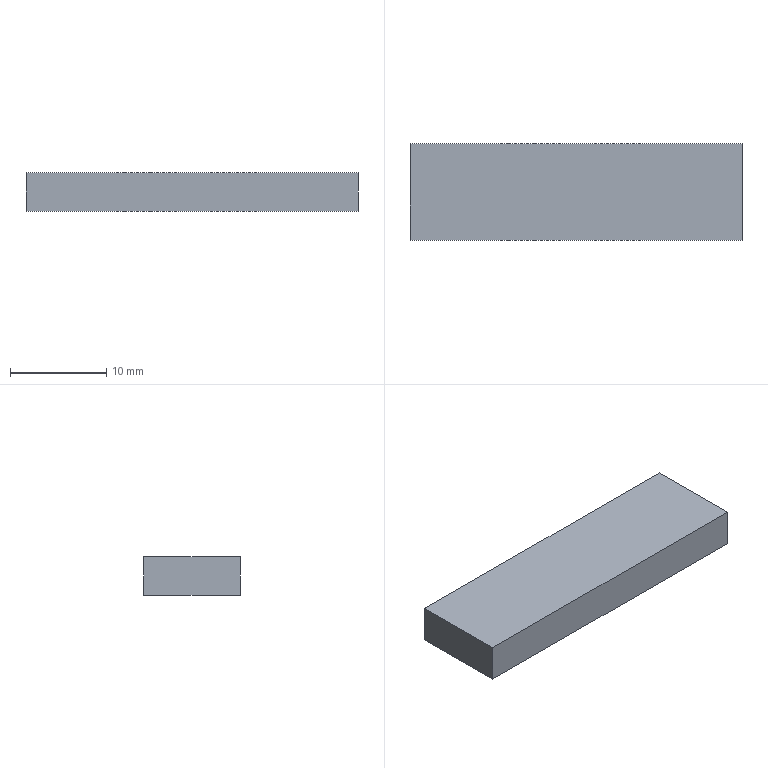Part | STEP file | YBQDJ-YB-30 | 1 solid | 6 faces | box 34.5 x 10 x 4 mm | volume 1380 mm3 | plane 6
STEP:
#1=CARTESIAN_POINT('',(0.,0.,0.));
#2=DIRECTION('',(0.,0.,1.));
#3=DIRECTION('',(1.,0.,0.));
#4=AXIS2_PLACEMENT_3D('',#1,#2,#3);
#5=CARTESIAN_POINT('',(-200.75,-276.,207.8));
#6=VERTEX_POINT('',#5);
#7=CARTESIAN_POINT('',(-200.75,-286.,207.8));
#8=VERTEX_POINT('',#7);
#9=CARTESIAN_POINT('',(-200.75,-276.,207.8));
#10=DIRECTION('',(0.,-1.,0.));
#11=VECTOR('',#10,1.);
#12=LINE('',#9,#11);
#13=CARTESIAN_POINT('',(-200.75,-276.,203.8));
#14=DIRECTION('',(-1.,0.,0.));
#15=DIRECTION('',(0.,0.,1.));
#16=AXIS2_PLACEMENT_3D('',#13,#14,#15);
#17=PLANE('',#16);
#18=CARTESIAN_POINT('',(4.,0.));
#19=DIRECTION('',(0.,-1.));
#20=VECTOR('',#19,1.);
#21=LINE('',#18,#20);
#22=(GEOMETRIC_REPRESENTATION_CONTEXT(2)PARAMETRIC_REPRESENTATION_CONTEXT()REPRESENTATION_CONTEXT('',''));
#23=DEFINITIONAL_REPRESENTATION('',(#21),#22);
#24=PCURVE('',#17,#23);
#25=CARTESIAN_POINT('',(0.,-172.,207.8));
#26=DIRECTION('',(0.,0.,1.));
#27=DIRECTION('',(1.,0.,0.));
#28=AXIS2_PLACEMENT_3D('',#25,#26,#27);
#29=PLANE('',#28);
#30=CARTESIAN_POINT('',(-200.75,-104.));
#31=DIRECTION('',(0.,-1.));
#32=VECTOR('',#31,1.);
#33=LINE('',#30,#32);
#34=(GEOMETRIC_REPRESENTATION_CONTEXT(2)PARAMETRIC_REPRESENTATION_CONTEXT()REPRESENTATION_CONTEXT('',''));
#35=DEFINITIONAL_REPRESENTATION('',(#33),#34);
#36=PCURVE('',#29,#35);
#37=SURFACE_CURVE('',#12,(#24,#36),.PCURVE_S1.);
#38=EDGE_CURVE('',#6,#8,#37,.T.);
#39=ORIENTED_EDGE('',*,*,#38,.F.);
#40=CARTESIAN_POINT('',(-200.75,-276.,203.8));
#41=VERTEX_POINT('',#40);
#42=CARTESIAN_POINT('',(-200.75,-276.,203.8));
#43=DIRECTION('',(0.,0.,1.));
#44=VECTOR('',#43,1.);
#45=LINE('',#42,#44);
#46=CARTESIAN_POINT('',(0.,0.));
#47=DIRECTION('',(1.,0.));
#48=VECTOR('',#47,1.);
#49=LINE('',#46,#48);
#50=(GEOMETRIC_REPRESENTATION_CONTEXT(2)PARAMETRIC_REPRESENTATION_CONTEXT()REPRESENTATION_CONTEXT('',''));
#51=DEFINITIONAL_REPRESENTATION('',(#49),#50);
#52=PCURVE('',#17,#51);
#53=CARTESIAN_POINT('',(-166.25,-276.,203.8));
#54=DIRECTION('',(0.,1.,0.));
#55=DIRECTION('',(0.,0.,1.));
#56=AXIS2_PLACEMENT_3D('',#53,#54,#55);
#57=PLANE('',#56);
#58=CARTESIAN_POINT('',(0.,-34.5));
#59=DIRECTION('',(1.,0.));
#60=VECTOR('',#59,1.);
#61=LINE('',#58,#60);
#62=(GEOMETRIC_REPRESENTATION_CONTEXT(2)PARAMETRIC_REPRESENTATION_CONTEXT()REPRESENTATION_CONTEXT('',''));
#63=DEFINITIONAL_REPRESENTATION('',(#61),#62);
#64=PCURVE('',#57,#63);
#65=SURFACE_CURVE('',#45,(#52,#64),.PCURVE_S1.);
#66=EDGE_CURVE('',#41,#6,#65,.T.);
#67=ORIENTED_EDGE('',*,*,#66,.F.);
#68=CARTESIAN_POINT('',(-200.75,-286.,203.8));
#69=VERTEX_POINT('',#68);
#70=CARTESIAN_POINT('',(-200.75,-276.,203.8));
#71=DIRECTION('',(0.,-1.,0.));
#72=VECTOR('',#71,1.);
#73=LINE('',#70,#72);
#74=CARTESIAN_POINT('',(0.,0.));
#75=DIRECTION('',(0.,-1.));
#76=VECTOR('',#75,1.);
#77=LINE('',#74,#76);
#78=(GEOMETRIC_REPRESENTATION_CONTEXT(2)PARAMETRIC_REPRESENTATION_CONTEXT()REPRESENTATION_CONTEXT('',''));
#79=DEFINITIONAL_REPRESENTATION('',(#77),#78);
#80=PCURVE('',#17,#79);
#81=CARTESIAN_POINT('',(0.,-172.,203.8));
#82=DIRECTION('',(0.,0.,1.));
#83=DIRECTION('',(1.,0.,0.));
#84=AXIS2_PLACEMENT_3D('',#81,#82,#83);
#85=PLANE('',#84);
#86=CARTESIAN_POINT('',(-200.75,-104.));
#87=DIRECTION('',(0.,-1.));
#88=VECTOR('',#87,1.);
#89=LINE('',#86,#88);
#90=(GEOMETRIC_REPRESENTATION_CONTEXT(2)PARAMETRIC_REPRESENTATION_CONTEXT()REPRESENTATION_CONTEXT('',''));
#91=DEFINITIONAL_REPRESENTATION('',(#89),#90);
#92=PCURVE('',#85,#91);
#93=SURFACE_CURVE('',#73,(#80,#92),.PCURVE_S1.);
#94=EDGE_CURVE('',#41,#69,#93,.T.);
#95=ORIENTED_EDGE('',*,*,#94,.T.);
#96=CARTESIAN_POINT('',(-200.75,-286.,203.8));
#97=DIRECTION('',(0.,0.,1.));
#98=VECTOR('',#97,1.);
#99=LINE('',#96,#98);
#100=CARTESIAN_POINT('',(0.,-10.));
#101=DIRECTION('',(1.,0.));
#102=VECTOR('',#101,1.);
#103=LINE('',#100,#102);
#104=(GEOMETRIC_REPRESENTATION_CONTEXT(2)PARAMETRIC_REPRESENTATION_CONTEXT()REPRESENTATION_CONTEXT('',''));
#105=DEFINITIONAL_REPRESENTATION('',(#103),#104);
#106=PCURVE('',#17,#105);
#107=CARTESIAN_POINT('',(-200.75,-286.,203.8));
#108=DIRECTION('',(0.,-1.,0.));
#109=DIRECTION('',(0.,0.,-1.));
#110=AXIS2_PLACEMENT_3D('',#107,#108,#109);
#111=PLANE('',#110);
#112=CARTESIAN_POINT('',(0.,0.));
#113=DIRECTION('',(-1.,0.));
#114=VECTOR('',#113,1.);
#115=LINE('',#112,#114);
#116=(GEOMETRIC_REPRESENTATION_CONTEXT(2)PARAMETRIC_REPRESENTATION_CONTEXT()REPRESENTATION_CONTEXT('',''));
#117=DEFINITIONAL_REPRESENTATION('',(#115),#116);
#118=PCURVE('',#111,#117);
#119=SURFACE_CURVE('',#99,(#106,#118),.PCURVE_S1.);
#120=EDGE_CURVE('',#69,#8,#119,.T.);
#121=ORIENTED_EDGE('',*,*,#120,.T.);
#122=EDGE_LOOP('',(#39,#67,#95,#121));
#123=FACE_BOUND('',#122,.T.);
#124=ADVANCED_FACE('',(#123),#17,.T.);
#125=CARTESIAN_POINT('',(-166.25,-286.,207.8));
#126=VERTEX_POINT('',#125);
#127=CARTESIAN_POINT('',(-200.75,-286.,207.8));
#128=DIRECTION('',(1.,0.,0.));
#129=VECTOR('',#128,1.);
#130=LINE('',#127,#129);
#131=CARTESIAN_POINT('',(-4.,0.));
#132=DIRECTION('',(0.,1.));
#133=VECTOR('',#132,1.);
#134=LINE('',#131,#133);
#135=(GEOMETRIC_REPRESENTATION_CONTEXT(2)PARAMETRIC_REPRESENTATION_CONTEXT()REPRESENTATION_CONTEXT('',''));
#136=DEFINITIONAL_REPRESENTATION('',(#134),#135);
#137=PCURVE('',#111,#136);
#138=CARTESIAN_POINT('',(-200.75,-114.));
#139=DIRECTION('',(1.,0.));
#140=VECTOR('',#139,1.);
#141=LINE('',#138,#140);
#142=(GEOMETRIC_REPRESENTATION_CONTEXT(2)PARAMETRIC_REPRESENTATION_CONTEXT()REPRESENTATION_CONTEXT('',''));
#143=DEFINITIONAL_REPRESENTATION('',(#141),#142);
#144=PCURVE('',#29,#143);
#145=SURFACE_CURVE('',#130,(#137,#144),.PCURVE_S1.);
#146=EDGE_CURVE('',#8,#126,#145,.T.);
#147=ORIENTED_EDGE('',*,*,#146,.F.);
#148=ORIENTED_EDGE('',*,*,#120,.F.);
#149=CARTESIAN_POINT('',(-166.25,-286.,203.8));
#150=VERTEX_POINT('',#149);
#151=CARTESIAN_POINT('',(-200.75,-286.,203.8));
#152=DIRECTION('',(1.,0.,0.));
#153=VECTOR('',#152,1.);
#154=LINE('',#151,#153);
#155=CARTESIAN_POINT('',(0.,0.));
#156=DIRECTION('',(0.,1.));
#157=VECTOR('',#156,1.);
#158=LINE('',#155,#157);
#159=(GEOMETRIC_REPRESENTATION_CONTEXT(2)PARAMETRIC_REPRESENTATION_CONTEXT()REPRESENTATION_CONTEXT('',''));
#160=DEFINITIONAL_REPRESENTATION('',(#158),#159);
#161=PCURVE('',#111,#160);
#162=CARTESIAN_POINT('',(-200.75,-114.));
#163=DIRECTION('',(1.,0.));
#164=VECTOR('',#163,1.);
#165=LINE('',#162,#164);
#166=(GEOMETRIC_REPRESENTATION_CONTEXT(2)PARAMETRIC_REPRESENTATION_CONTEXT()REPRESENTATION_CONTEXT('',''));
#167=DEFINITIONAL_REPRESENTATION('',(#165),#166);
#168=PCURVE('',#85,#167);
#169=SURFACE_CURVE('',#154,(#161,#168),.PCURVE_S1.);
#170=EDGE_CURVE('',#69,#150,#169,.T.);
#171=ORIENTED_EDGE('',*,*,#170,.T.);
#172=CARTESIAN_POINT('',(-166.25,-286.,203.8));
#173=DIRECTION('',(0.,0.,1.));
#174=VECTOR('',#173,1.);
#175=LINE('',#172,#174);
#176=CARTESIAN_POINT('',(0.,34.5));
#177=DIRECTION('',(-1.,0.));
#178=VECTOR('',#177,1.);
#179=LINE('',#176,#178);
#180=(GEOMETRIC_REPRESENTATION_CONTEXT(2)PARAMETRIC_REPRESENTATION_CONTEXT()REPRESENTATION_CONTEXT('',''));
#181=DEFINITIONAL_REPRESENTATION('',(#179),#180);
#182=PCURVE('',#111,#181);
#183=CARTESIAN_POINT('',(-166.25,-286.,203.8));
#184=DIRECTION('',(1.,0.,0.));
#185=DIRECTION('',(0.,0.,-1.));
#186=AXIS2_PLACEMENT_3D('',#183,#184,#185);
#187=PLANE('',#186);
#188=CARTESIAN_POINT('',(0.,0.));
#189=DIRECTION('',(-1.,0.));
#190=VECTOR('',#189,1.);
#191=LINE('',#188,#190);
#192=(GEOMETRIC_REPRESENTATION_CONTEXT(2)PARAMETRIC_REPRESENTATION_CONTEXT()REPRESENTATION_CONTEXT('',''));
#193=DEFINITIONAL_REPRESENTATION('',(#191),#192);
#194=PCURVE('',#187,#193);
#195=SURFACE_CURVE('',#175,(#182,#194),.PCURVE_S1.);
#196=EDGE_CURVE('',#150,#126,#195,.T.);
#197=ORIENTED_EDGE('',*,*,#196,.T.);
#198=EDGE_LOOP('',(#147,#148,#171,#197));
#199=FACE_BOUND('',#198,.T.);
#200=ADVANCED_FACE('',(#199),#111,.T.);
#201=CARTESIAN_POINT('',(-166.25,-276.,207.8));
#202=VERTEX_POINT('',#201);
#203=CARTESIAN_POINT('',(-166.25,-286.,207.8));
#204=DIRECTION('',(0.,1.,0.));
#205=VECTOR('',#204,1.);
#206=LINE('',#203,#205);
#207=CARTESIAN_POINT('',(-4.,0.));
#208=DIRECTION('',(0.,1.));
#209=VECTOR('',#208,1.);
#210=LINE('',#207,#209);
#211=(GEOMETRIC_REPRESENTATION_CONTEXT(2)PARAMETRIC_REPRESENTATION_CONTEXT()REPRESENTATION_CONTEXT('',''));
#212=DEFINITIONAL_REPRESENTATION('',(#210),#211);
#213=PCURVE('',#187,#212);
#214=CARTESIAN_POINT('',(-166.25,-114.));
#215=DIRECTION('',(0.,1.));
#216=VECTOR('',#215,1.);
#217=LINE('',#214,#216);
#218=(GEOMETRIC_REPRESENTATION_CONTEXT(2)PARAMETRIC_REPRESENTATION_CONTEXT()REPRESENTATION_CONTEXT('',''));
#219=DEFINITIONAL_REPRESENTATION('',(#217),#218);
#220=PCURVE('',#29,#219);
#221=SURFACE_CURVE('',#206,(#213,#220),.PCURVE_S1.);
#222=EDGE_CURVE('',#126,#202,#221,.T.);
#223=ORIENTED_EDGE('',*,*,#222,.F.);
#224=ORIENTED_EDGE('',*,*,#196,.F.);
#225=CARTESIAN_POINT('',(-166.25,-276.,203.8));
#226=VERTEX_POINT('',#225);
#227=CARTESIAN_POINT('',(-166.25,-286.,203.8));
#228=DIRECTION('',(0.,1.,0.));
#229=VECTOR('',#228,1.);
#230=LINE('',#227,#229);
#231=CARTESIAN_POINT('',(0.,0.));
#232=DIRECTION('',(0.,1.));
#233=VECTOR('',#232,1.);
#234=LINE('',#231,#233);
#235=(GEOMETRIC_REPRESENTATION_CONTEXT(2)PARAMETRIC_REPRESENTATION_CONTEXT()REPRESENTATION_CONTEXT('',''));
#236=DEFINITIONAL_REPRESENTATION('',(#234),#235);
#237=PCURVE('',#187,#236);
#238=CARTESIAN_POINT('',(-166.25,-114.));
#239=DIRECTION('',(0.,1.));
#240=VECTOR('',#239,1.);
#241=LINE('',#238,#240);
#242=(GEOMETRIC_REPRESENTATION_CONTEXT(2)PARAMETRIC_REPRESENTATION_CONTEXT()REPRESENTATION_CONTEXT('',''));
#243=DEFINITIONAL_REPRESENTATION('',(#241),#242);
#244=PCURVE('',#85,#243);
#245=SURFACE_CURVE('',#230,(#237,#244),.PCURVE_S1.);
#246=EDGE_CURVE('',#150,#226,#245,.T.);
#247=ORIENTED_EDGE('',*,*,#246,.T.);
#248=CARTESIAN_POINT('',(-166.25,-276.,203.8));
#249=DIRECTION('',(0.,0.,1.));
#250=VECTOR('',#249,1.);
#251=LINE('',#248,#250);
#252=CARTESIAN_POINT('',(0.,10.));
#253=DIRECTION('',(-1.,0.));
#254=VECTOR('',#253,1.);
#255=LINE('',#252,#254);
#256=(GEOMETRIC_REPRESENTATION_CONTEXT(2)PARAMETRIC_REPRESENTATION_CONTEXT()REPRESENTATION_CONTEXT('',''));
#257=DEFINITIONAL_REPRESENTATION('',(#255),#256);
#258=PCURVE('',#187,#257);
#259=CARTESIAN_POINT('',(0.,0.));
#260=DIRECTION('',(1.,0.));
#261=VECTOR('',#260,1.);
#262=LINE('',#259,#261);
#263=(GEOMETRIC_REPRESENTATION_CONTEXT(2)PARAMETRIC_REPRESENTATION_CONTEXT()REPRESENTATION_CONTEXT('',''));
#264=DEFINITIONAL_REPRESENTATION('',(#262),#263);
#265=PCURVE('',#57,#264);
#266=SURFACE_CURVE('',#251,(#258,#265),.PCURVE_S1.);
#267=EDGE_CURVE('',#226,#202,#266,.T.);
#268=ORIENTED_EDGE('',*,*,#267,.T.);
#269=EDGE_LOOP('',(#223,#224,#247,#268));
#270=FACE_BOUND('',#269,.T.);
#271=ADVANCED_FACE('',(#270),#187,.T.);
#272=CARTESIAN_POINT('',(-166.25,-276.,207.8));
#273=DIRECTION('',(-1.,0.,0.));
#274=VECTOR('',#273,1.);
#275=LINE('',#272,#274);
#276=CARTESIAN_POINT('',(4.,0.));
#277=DIRECTION('',(0.,-1.));
#278=VECTOR('',#277,1.);
#279=LINE('',#276,#278);
#280=(GEOMETRIC_REPRESENTATION_CONTEXT(2)PARAMETRIC_REPRESENTATION_CONTEXT()REPRESENTATION_CONTEXT('',''));
#281=DEFINITIONAL_REPRESENTATION('',(#279),#280);
#282=PCURVE('',#57,#281);
#283=CARTESIAN_POINT('',(-166.25,-104.));
#284=DIRECTION('',(-1.,0.));
#285=VECTOR('',#284,1.);
#286=LINE('',#283,#285);
#287=(GEOMETRIC_REPRESENTATION_CONTEXT(2)PARAMETRIC_REPRESENTATION_CONTEXT()REPRESENTATION_CONTEXT('',''));
#288=DEFINITIONAL_REPRESENTATION('',(#286),#287);
#289=PCURVE('',#29,#288);
#290=SURFACE_CURVE('',#275,(#282,#289),.PCURVE_S1.);
#291=EDGE_CURVE('',#202,#6,#290,.T.);
#292=ORIENTED_EDGE('',*,*,#291,.F.);
#293=ORIENTED_EDGE('',*,*,#267,.F.);
#294=CARTESIAN_POINT('',(-166.25,-276.,203.8));
#295=DIRECTION('',(-1.,0.,0.));
#296=VECTOR('',#295,1.);
#297=LINE('',#294,#296);
#298=CARTESIAN_POINT('',(0.,0.));
#299=DIRECTION('',(0.,-1.));
#300=VECTOR('',#299,1.);
#301=LINE('',#298,#300);
#302=(GEOMETRIC_REPRESENTATION_CONTEXT(2)PARAMETRIC_REPRESENTATION_CONTEXT()REPRESENTATION_CONTEXT('',''));
#303=DEFINITIONAL_REPRESENTATION('',(#301),#302);
#304=PCURVE('',#57,#303);
#305=CARTESIAN_POINT('',(-166.25,-104.));
#306=DIRECTION('',(-1.,0.));
#307=VECTOR('',#306,1.);
#308=LINE('',#305,#307);
#309=(GEOMETRIC_REPRESENTATION_CONTEXT(2)PARAMETRIC_REPRESENTATION_CONTEXT()REPRESENTATION_CONTEXT('',''));
#310=DEFINITIONAL_REPRESENTATION('',(#308),#309);
#311=PCURVE('',#85,#310);
#312=SURFACE_CURVE('',#297,(#304,#311),.PCURVE_S1.);
#313=EDGE_CURVE('',#226,#41,#312,.T.);
#314=ORIENTED_EDGE('',*,*,#313,.T.);
#315=ORIENTED_EDGE('',*,*,#66,.T.);
#316=EDGE_LOOP('',(#292,#293,#314,#315));
#317=FACE_BOUND('',#316,.T.);
#318=ADVANCED_FACE('',(#317),#57,.T.);
#319=ORIENTED_EDGE('',*,*,#94,.F.);
#320=ORIENTED_EDGE('',*,*,#313,.F.);
#321=ORIENTED_EDGE('',*,*,#246,.F.);
#322=ORIENTED_EDGE('',*,*,#170,.F.);
#323=EDGE_LOOP('',(#319,#320,#321,#322));
#324=FACE_BOUND('',#323,.T.);
#325=ADVANCED_FACE('',(#324),#85,.F.);
#326=ORIENTED_EDGE('',*,*,#38,.T.);
#327=ORIENTED_EDGE('',*,*,#146,.T.);
#328=ORIENTED_EDGE('',*,*,#222,.T.);
#329=ORIENTED_EDGE('',*,*,#291,.T.);
#330=EDGE_LOOP('',(#326,#327,#328,#329));
#331=FACE_BOUND('',#330,.T.);
#332=ADVANCED_FACE('',(#331),#29,.T.);
#333=CLOSED_SHELL('',(#124,#200,#271,#318,#325,#332));
#334=MANIFOLD_SOLID_BREP('',#333);
#335=(LENGTH_UNIT()NAMED_UNIT(*)SI_UNIT(.MILLI.,.METRE.));
#336=UNCERTAINTY_MEASURE_WITH_UNIT(LENGTH_MEASURE(0.0000001),#335,'','');
#337=(NAMED_UNIT(*)PLANE_ANGLE_UNIT()SI_UNIT($,.RADIAN.));
#338=(NAMED_UNIT(*)SI_UNIT($,.STERADIAN.)SOLID_ANGLE_UNIT());
#339=(GEOMETRIC_REPRESENTATION_CONTEXT(3)GLOBAL_UNCERTAINTY_ASSIGNED_CONTEXT((#336))GLOBAL_UNIT_ASSIGNED_CONTEXT((#335,#337,#338))REPRESENTATION_CONTEXT('',''));
#340=ADVANCED_BREP_SHAPE_REPRESENTATION('',(#4,#334),#339);